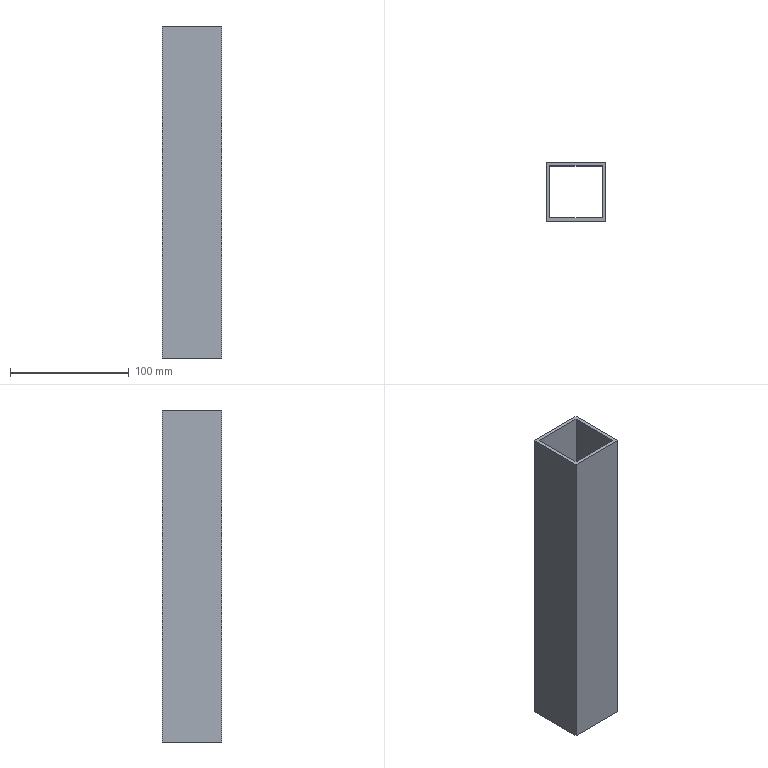Part | SolidWorks | features Extrusion 1 | 1 solid | 10 faces | box 50 x 50 x 280 mm | volume 157920 mm3 | plane 10
STEP:
#1=CARTESIAN_POINT('',(0.,0.,280.));
#2=VERTEX_POINT('',#1);
#3=CARTESIAN_POINT('',(50.,0.,280.));
#4=VERTEX_POINT('',#3);
#5=CARTESIAN_POINT('',(50.,0.,280.));
#6=DIRECTION('',(1.,0.,0.));
#7=VECTOR('',#6,1000.);
#8=LINE('',#5,#7);
#9=EDGE_CURVE('',#2,#4,#8,.T.);
#10=ORIENTED_EDGE('',*,*,#9,.T.);
#11=CARTESIAN_POINT('',(50.,50.,280.));
#12=VERTEX_POINT('',#11);
#13=CARTESIAN_POINT('',(50.,50.,280.));
#14=DIRECTION('',(0.,1.,0.));
#15=VECTOR('',#14,1000.);
#16=LINE('',#13,#15);
#17=EDGE_CURVE('',#4,#12,#16,.T.);
#18=ORIENTED_EDGE('',*,*,#17,.T.);
#19=CARTESIAN_POINT('',(0.,50.,280.));
#20=VERTEX_POINT('',#19);
#21=CARTESIAN_POINT('',(0.,50.,280.));
#22=DIRECTION('',(-1.,0.,0.));
#23=VECTOR('',#22,1000.);
#24=LINE('',#21,#23);
#25=EDGE_CURVE('',#12,#20,#24,.T.);
#26=ORIENTED_EDGE('',*,*,#25,.T.);
#27=CARTESIAN_POINT('',(0.,0.,280.));
#28=DIRECTION('',(0.,-1.,0.));
#29=VECTOR('',#28,1000.);
#30=LINE('',#27,#29);
#31=EDGE_CURVE('',#20,#2,#30,.T.);
#32=ORIENTED_EDGE('',*,*,#31,.T.);
#33=EDGE_LOOP('',(#10,#18,#26,#32));
#34=FACE_OUTER_BOUND('',#33,.T.);
#35=CARTESIAN_POINT('',(3.,3.,280.));
#36=VERTEX_POINT('',#35);
#37=CARTESIAN_POINT('',(47.,3.,280.));
#38=VERTEX_POINT('',#37);
#39=CARTESIAN_POINT('',(47.,3.,280.));
#40=DIRECTION('',(1.,0.,0.));
#41=VECTOR('',#40,1000.);
#42=LINE('',#39,#41);
#43=EDGE_CURVE('',#36,#38,#42,.T.);
#44=ORIENTED_EDGE('',*,*,#43,.F.);
#45=CARTESIAN_POINT('',(3.,47.,280.));
#46=VERTEX_POINT('',#45);
#47=CARTESIAN_POINT('',(3.,3.,280.));
#48=DIRECTION('',(0.,-1.,0.));
#49=VECTOR('',#48,1000.);
#50=LINE('',#47,#49);
#51=EDGE_CURVE('',#46,#36,#50,.T.);
#52=ORIENTED_EDGE('',*,*,#51,.F.);
#53=CARTESIAN_POINT('',(47.,47.,280.));
#54=VERTEX_POINT('',#53);
#55=CARTESIAN_POINT('',(3.,47.,280.));
#56=DIRECTION('',(-1.,0.,0.));
#57=VECTOR('',#56,1000.);
#58=LINE('',#55,#57);
#59=EDGE_CURVE('',#54,#46,#58,.T.);
#60=ORIENTED_EDGE('',*,*,#59,.F.);
#61=CARTESIAN_POINT('',(47.,47.,280.));
#62=DIRECTION('',(0.,1.,0.));
#63=VECTOR('',#62,1000.);
#64=LINE('',#61,#63);
#65=EDGE_CURVE('',#38,#54,#64,.T.);
#66=ORIENTED_EDGE('',*,*,#65,.F.);
#67=EDGE_LOOP('',(#44,#52,#60,#66));
#68=FACE_BOUND('',#67,.T.);
#69=CARTESIAN_POINT('',(0.,0.,280.));
#70=DIRECTION('',(0.,0.,-1.));
#71=DIRECTION('',(-1.,0.,0.));
#72=AXIS2_PLACEMENT_3D('',#69,#70,#71);
#73=PLANE('',#72);
#74=ADVANCED_FACE('',(#34,#68),#73,.F.);
#75=CARTESIAN_POINT('',(0.,0.,0.));
#76=VERTEX_POINT('',#75);
#77=CARTESIAN_POINT('',(50.,0.,0.));
#78=VERTEX_POINT('',#77);
#79=CARTESIAN_POINT('',(50.,0.,0.));
#80=DIRECTION('',(1.,0.,0.));
#81=VECTOR('',#80,1000.);
#82=LINE('',#79,#81);
#83=EDGE_CURVE('',#76,#78,#82,.T.);
#84=ORIENTED_EDGE('',*,*,#83,.F.);
#85=CARTESIAN_POINT('',(0.,50.,0.));
#86=VERTEX_POINT('',#85);
#87=CARTESIAN_POINT('',(0.,0.,0.));
#88=DIRECTION('',(0.,-1.,0.));
#89=VECTOR('',#88,1000.);
#90=LINE('',#87,#89);
#91=EDGE_CURVE('',#86,#76,#90,.T.);
#92=ORIENTED_EDGE('',*,*,#91,.F.);
#93=CARTESIAN_POINT('',(50.,50.,0.));
#94=VERTEX_POINT('',#93);
#95=CARTESIAN_POINT('',(0.,50.,0.));
#96=DIRECTION('',(-1.,0.,0.));
#97=VECTOR('',#96,1000.);
#98=LINE('',#95,#97);
#99=EDGE_CURVE('',#94,#86,#98,.T.);
#100=ORIENTED_EDGE('',*,*,#99,.F.);
#101=CARTESIAN_POINT('',(50.,50.,0.));
#102=DIRECTION('',(0.,1.,0.));
#103=VECTOR('',#102,1000.);
#104=LINE('',#101,#103);
#105=EDGE_CURVE('',#78,#94,#104,.T.);
#106=ORIENTED_EDGE('',*,*,#105,.F.);
#107=EDGE_LOOP('',(#84,#92,#100,#106));
#108=FACE_OUTER_BOUND('',#107,.T.);
#109=CARTESIAN_POINT('',(3.,47.,0.));
#110=VERTEX_POINT('',#109);
#111=CARTESIAN_POINT('',(3.,3.,0.));
#112=VERTEX_POINT('',#111);
#113=CARTESIAN_POINT('',(3.,3.,0.));
#114=DIRECTION('',(0.,-1.,0.));
#115=VECTOR('',#114,1000.);
#116=LINE('',#113,#115);
#117=EDGE_CURVE('',#110,#112,#116,.T.);
#118=ORIENTED_EDGE('',*,*,#117,.T.);
#119=CARTESIAN_POINT('',(47.,3.,0.));
#120=VERTEX_POINT('',#119);
#121=CARTESIAN_POINT('',(47.,3.,0.));
#122=DIRECTION('',(1.,0.,0.));
#123=VECTOR('',#122,1000.);
#124=LINE('',#121,#123);
#125=EDGE_CURVE('',#112,#120,#124,.T.);
#126=ORIENTED_EDGE('',*,*,#125,.T.);
#127=CARTESIAN_POINT('',(47.,47.,0.));
#128=VERTEX_POINT('',#127);
#129=CARTESIAN_POINT('',(47.,47.,0.));
#130=DIRECTION('',(0.,1.,0.));
#131=VECTOR('',#130,1000.);
#132=LINE('',#129,#131);
#133=EDGE_CURVE('',#120,#128,#132,.T.);
#134=ORIENTED_EDGE('',*,*,#133,.T.);
#135=CARTESIAN_POINT('',(3.,47.,0.));
#136=DIRECTION('',(-1.,0.,0.));
#137=VECTOR('',#136,1000.);
#138=LINE('',#135,#137);
#139=EDGE_CURVE('',#128,#110,#138,.T.);
#140=ORIENTED_EDGE('',*,*,#139,.T.);
#141=EDGE_LOOP('',(#118,#126,#134,#140));
#142=FACE_BOUND('',#141,.T.);
#143=CARTESIAN_POINT('',(0.,0.,0.));
#144=DIRECTION('',(0.,0.,-1.));
#145=DIRECTION('',(-1.,0.,0.));
#146=AXIS2_PLACEMENT_3D('',#143,#144,#145);
#147=PLANE('',#146);
#148=ADVANCED_FACE('',(#108,#142),#147,.T.);
#149=ORIENTED_EDGE('',*,*,#83,.T.);
#150=CARTESIAN_POINT('',(50.,0.,280.));
#151=DIRECTION('',(0.,0.,-1.));
#152=VECTOR('',#151,1000.);
#153=LINE('',#150,#152);
#154=EDGE_CURVE('',#4,#78,#153,.T.);
#155=ORIENTED_EDGE('',*,*,#154,.F.);
#156=ORIENTED_EDGE('',*,*,#9,.F.);
#157=CARTESIAN_POINT('',(0.,0.,280.));
#158=DIRECTION('',(0.,0.,-1.));
#159=VECTOR('',#158,1000.);
#160=LINE('',#157,#159);
#161=EDGE_CURVE('',#2,#76,#160,.T.);
#162=ORIENTED_EDGE('',*,*,#161,.T.);
#163=EDGE_LOOP('',(#149,#155,#156,#162));
#164=FACE_OUTER_BOUND('',#163,.T.);
#165=CARTESIAN_POINT('',(50.,0.,280.));
#166=DIRECTION('',(0.,1.,0.));
#167=DIRECTION('',(0.,0.,1.));
#168=AXIS2_PLACEMENT_3D('',#165,#166,#167);
#169=PLANE('',#168);
#170=ADVANCED_FACE('',(#164),#169,.F.);
#171=ORIENTED_EDGE('',*,*,#105,.T.);
#172=CARTESIAN_POINT('',(50.,50.,280.));
#173=DIRECTION('',(0.,0.,-1.));
#174=VECTOR('',#173,1000.);
#175=LINE('',#172,#174);
#176=EDGE_CURVE('',#12,#94,#175,.T.);
#177=ORIENTED_EDGE('',*,*,#176,.F.);
#178=ORIENTED_EDGE('',*,*,#17,.F.);
#179=ORIENTED_EDGE('',*,*,#154,.T.);
#180=EDGE_LOOP('',(#171,#177,#178,#179));
#181=FACE_OUTER_BOUND('',#180,.T.);
#182=CARTESIAN_POINT('',(50.,50.,280.));
#183=DIRECTION('',(-1.,0.,0.));
#184=DIRECTION('',(0.,0.,1.));
#185=AXIS2_PLACEMENT_3D('',#182,#183,#184);
#186=PLANE('',#185);
#187=ADVANCED_FACE('',(#181),#186,.F.);
#188=ORIENTED_EDGE('',*,*,#99,.T.);
#189=CARTESIAN_POINT('',(0.,50.,280.));
#190=DIRECTION('',(0.,0.,-1.));
#191=VECTOR('',#190,1000.);
#192=LINE('',#189,#191);
#193=EDGE_CURVE('',#20,#86,#192,.T.);
#194=ORIENTED_EDGE('',*,*,#193,.F.);
#195=ORIENTED_EDGE('',*,*,#25,.F.);
#196=ORIENTED_EDGE('',*,*,#176,.T.);
#197=EDGE_LOOP('',(#188,#194,#195,#196));
#198=FACE_OUTER_BOUND('',#197,.T.);
#199=CARTESIAN_POINT('',(0.,50.,280.));
#200=DIRECTION('',(0.,-1.,0.));
#201=DIRECTION('',(0.,0.,-1.));
#202=AXIS2_PLACEMENT_3D('',#199,#200,#201);
#203=PLANE('',#202);
#204=ADVANCED_FACE('',(#198),#203,.F.);
#205=ORIENTED_EDGE('',*,*,#91,.T.);
#206=ORIENTED_EDGE('',*,*,#161,.F.);
#207=ORIENTED_EDGE('',*,*,#31,.F.);
#208=ORIENTED_EDGE('',*,*,#193,.T.);
#209=EDGE_LOOP('',(#205,#206,#207,#208));
#210=FACE_OUTER_BOUND('',#209,.T.);
#211=CARTESIAN_POINT('',(0.,0.,280.));
#212=DIRECTION('',(1.,0.,0.));
#213=DIRECTION('',(0.,0.,-1.));
#214=AXIS2_PLACEMENT_3D('',#211,#212,#213);
#215=PLANE('',#214);
#216=ADVANCED_FACE('',(#210),#215,.F.);
#217=ORIENTED_EDGE('',*,*,#125,.F.);
#218=CARTESIAN_POINT('',(3.,3.,280.));
#219=DIRECTION('',(0.,0.,-1.));
#220=VECTOR('',#219,1000.);
#221=LINE('',#218,#220);
#222=EDGE_CURVE('',#36,#112,#221,.T.);
#223=ORIENTED_EDGE('',*,*,#222,.F.);
#224=ORIENTED_EDGE('',*,*,#43,.T.);
#225=CARTESIAN_POINT('',(47.,3.,280.));
#226=DIRECTION('',(0.,0.,-1.));
#227=VECTOR('',#226,1000.);
#228=LINE('',#225,#227);
#229=EDGE_CURVE('',#38,#120,#228,.T.);
#230=ORIENTED_EDGE('',*,*,#229,.T.);
#231=EDGE_LOOP('',(#217,#223,#224,#230));
#232=FACE_OUTER_BOUND('',#231,.T.);
#233=CARTESIAN_POINT('',(47.,3.,280.));
#234=DIRECTION('',(0.,1.,0.));
#235=DIRECTION('',(0.,0.,1.));
#236=AXIS2_PLACEMENT_3D('',#233,#234,#235);
#237=PLANE('',#236);
#238=ADVANCED_FACE('',(#232),#237,.T.);
#239=ORIENTED_EDGE('',*,*,#133,.F.);
#240=ORIENTED_EDGE('',*,*,#229,.F.);
#241=ORIENTED_EDGE('',*,*,#65,.T.);
#242=CARTESIAN_POINT('',(47.,47.,280.));
#243=DIRECTION('',(0.,0.,-1.));
#244=VECTOR('',#243,1000.);
#245=LINE('',#242,#244);
#246=EDGE_CURVE('',#54,#128,#245,.T.);
#247=ORIENTED_EDGE('',*,*,#246,.T.);
#248=EDGE_LOOP('',(#239,#240,#241,#247));
#249=FACE_OUTER_BOUND('',#248,.T.);
#250=CARTESIAN_POINT('',(47.,47.,280.));
#251=DIRECTION('',(-1.,0.,0.));
#252=DIRECTION('',(0.,0.,1.));
#253=AXIS2_PLACEMENT_3D('',#250,#251,#252);
#254=PLANE('',#253);
#255=ADVANCED_FACE('',(#249),#254,.T.);
#256=ORIENTED_EDGE('',*,*,#139,.F.);
#257=ORIENTED_EDGE('',*,*,#246,.F.);
#258=ORIENTED_EDGE('',*,*,#59,.T.);
#259=CARTESIAN_POINT('',(3.,47.,280.));
#260=DIRECTION('',(0.,0.,-1.));
#261=VECTOR('',#260,1000.);
#262=LINE('',#259,#261);
#263=EDGE_CURVE('',#46,#110,#262,.T.);
#264=ORIENTED_EDGE('',*,*,#263,.T.);
#265=EDGE_LOOP('',(#256,#257,#258,#264));
#266=FACE_OUTER_BOUND('',#265,.T.);
#267=CARTESIAN_POINT('',(3.,47.,280.));
#268=DIRECTION('',(0.,-1.,0.));
#269=DIRECTION('',(0.,0.,-1.));
#270=AXIS2_PLACEMENT_3D('',#267,#268,#269);
#271=PLANE('',#270);
#272=ADVANCED_FACE('',(#266),#271,.T.);
#273=ORIENTED_EDGE('',*,*,#117,.F.);
#274=ORIENTED_EDGE('',*,*,#263,.F.);
#275=ORIENTED_EDGE('',*,*,#51,.T.);
#276=ORIENTED_EDGE('',*,*,#222,.T.);
#277=EDGE_LOOP('',(#273,#274,#275,#276));
#278=FACE_OUTER_BOUND('',#277,.T.);
#279=CARTESIAN_POINT('',(3.,3.,280.));
#280=DIRECTION('',(1.,0.,0.));
#281=DIRECTION('',(0.,0.,-1.));
#282=AXIS2_PLACEMENT_3D('',#279,#280,#281);
#283=PLANE('',#282);
#284=ADVANCED_FACE('',(#278),#283,.T.);
#285=CLOSED_SHELL('',(#74,#148,#170,#187,#204,#216,#238,#255,#272,#284));
#286=MANIFOLD_SOLID_BREP('',#285);
#287=CARTESIAN_POINT('',(0.,0.,0.));
#288=DIRECTION('',(0.,0.,1.));
#289=DIRECTION('',(1.,0.,0.));
#290=AXIS2_PLACEMENT_3D('',#287,#288,#289);
#291=(LENGTH_UNIT()NAMED_UNIT(*)SI_UNIT(.MILLI.,.METRE.));
#292=UNCERTAINTY_MEASURE_WITH_UNIT(LENGTH_MEASURE(0.00001),#291,'','');
#293=(NAMED_UNIT(*)PLANE_ANGLE_UNIT()SI_UNIT($,.RADIAN.));
#294=(NAMED_UNIT(*)SI_UNIT($,.STERADIAN.)SOLID_ANGLE_UNIT());
#295=(GEOMETRIC_REPRESENTATION_CONTEXT(3)GLOBAL_UNCERTAINTY_ASSIGNED_CONTEXT((#292))GLOBAL_UNIT_ASSIGNED_CONTEXT((#291,#293,#294))REPRESENTATION_CONTEXT('',''));
#296=ADVANCED_BREP_SHAPE_REPRESENTATION('',(#286,#290),#295);